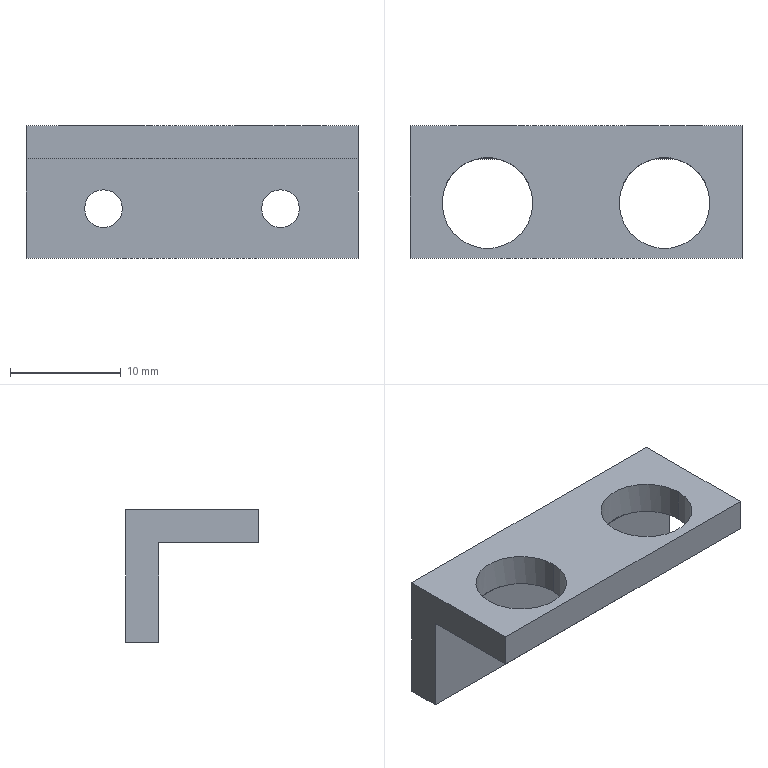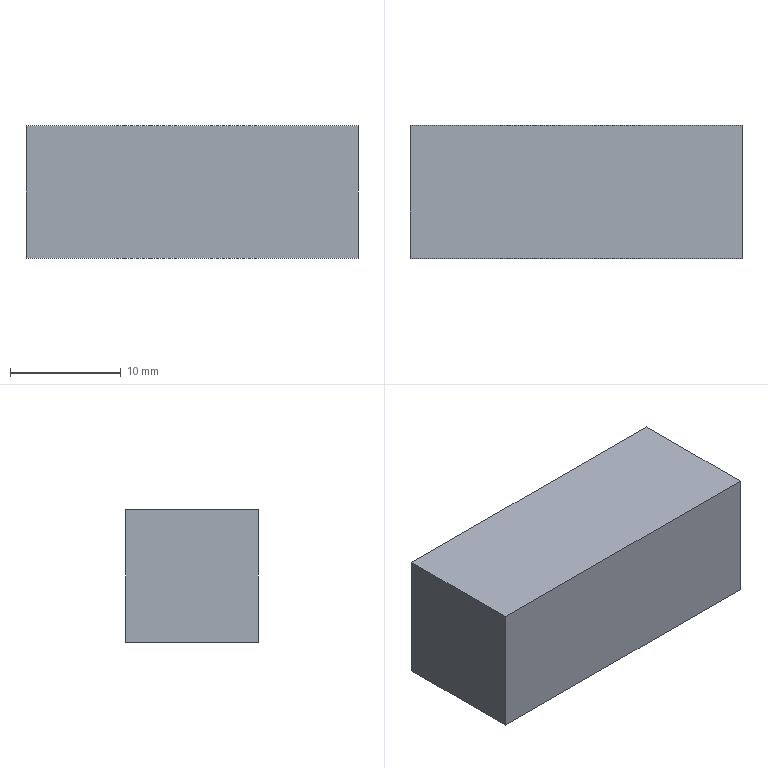CAM job | NX | 3+2 milling, drilling | part box 30 x 12 x 12 mm | stock box 30 x 12 x 12 mm
Tools:
number,name,description,diameter,corner_radius,flute_length,length,flutes
21,ZXZ,Milling Tool-5 Parameters,6.0,0.0,50.0,75.0,2
13,3.4ZT,Drilling Tool,3.4,0.0,35.0,50.0,2
7,D3R0.5,Milling Tool-5 Parameters,3.0,0.5,50.0,75.0,2
4,D10,Milling Tool-5 Parameters,10.0,0.0,50.0,75.0,2
17,D4,Milling Tool-5 Parameters,4.0,0.0,50.0,75.0,2
1,D6A45,Milling Tool-5 Parameters,6.0,0.0,50.0,75.0,2
14,D10JING,Milling Tool-5 Parameters,10.0,0.0,50.0,75.0,2
Operations:
program,operation,operation_type,tool,method,geometry_group,spindle_rpm,surface_speed,feed_per_tooth,feed_cut,feed_plunge,cut_length_mm,path_length_mm,cut_time_min,machine_time_min
1,DRILLING,Operation,ZXZ,METHOD,A,3500.0,65.0,0.0357,250.0,0.0,8.0,95.279,0.032,0.0407
1,DRILLING_COPY_1,Operation,3.4ZT,METHOD,A,2000.0,21.0,0.0375,150.0,0.0,17.043,113.365,0.1136,0.1233
1,ZLEVEL_PROFILE_1_1,ZLevelMilling,D3R0.5,METHOD,A,7500.0,94.0,0.1667,2500.0,1000.0,410.065,546.636,0.1664,0.1801
1,PLANAR_MILL_COPY_1_COPY_COPY,PlanarMilling,D6A45,METHOD,A,7500.0,141.0,0.0833,1250.0,100.0,95.4,153.4,0.0763,0.0821
2,HOLE_MILLING,CylinderMilling,D4,METHOD,B,5000.0,62.0,0.125,1250.0,100.0,1137.279,1278.279,0.9098,0.9239
2,PLANAR_MILL_COPY_1_COPY,PlanarMilling,D6A45,METHOD,B,7500.0,141.0,0.0833,1250.0,100.0,147.103,338.501,0.1177,0.1368
3,ZLEVEL_PROFILE,ZLevelMilling,D10,METHOD,C,3500.0,109.0,0.3143,2200.0,1000.0,1521.025,1599.068,0.7498,0.7576
3,FLOOR_WALL_1_COPY_COPY,VolumeBased25DMillingOperation,D10JING,METHOD,C,7500.0,235.0,0.08,1200.0,1000.0,44.0,120.0,0.0378,0.0454
3,PLANAR_MILL_COPY_1_COPY_COPY_COPY,PlanarMilling,D6A45,METHOD,C,7500.0,141.0,0.0833,1250.0,100.0,77.4,135.4,0.0619,0.0677
3,PLANAR_MILL_COPY_1_COPY_COPY_COPY_COPY,PlanarMilling,D6A45,METHOD,C,7500.0,141.0,0.0833,1250.0,100.0,81.813,360.056,0.0655,0.0933